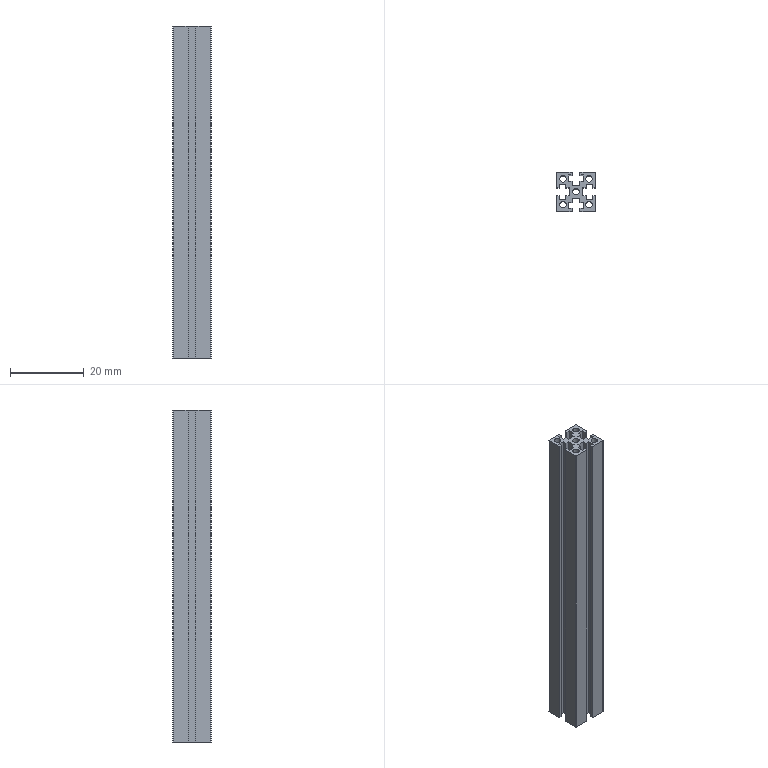Part | SolidWorks | features ICE 3, Extrusion 1, Scale 1 | 1 solid | 68 faces | box 10.5 x 10.5 x 90 mm | volume 4956 mm3 | plane 54 | cylinder 14 | commonest cylinder face diameters 1.75 x10 0.42 x4